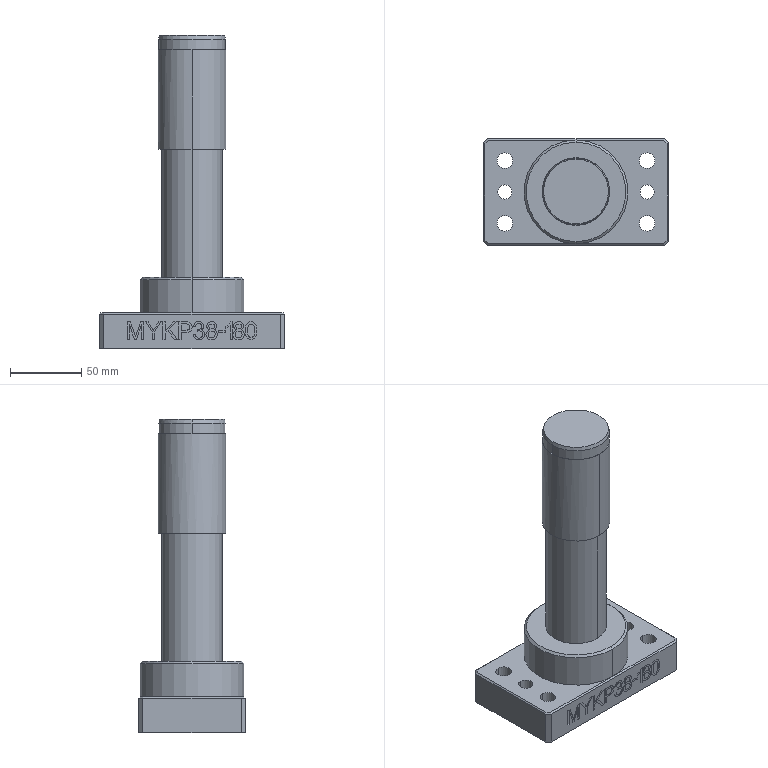Part | STEP file | PN_0058_id1510_x_t | 1 solid | 193 faces | box 130 x 75 x 220 mm | volume 598119 mm3 | plane 123 | cylinder 62 | cone 8 | commonest cylinder face diameters 11 x8 3.991 x4 4.986 x4 10 x4 38 x4 5.938 x2